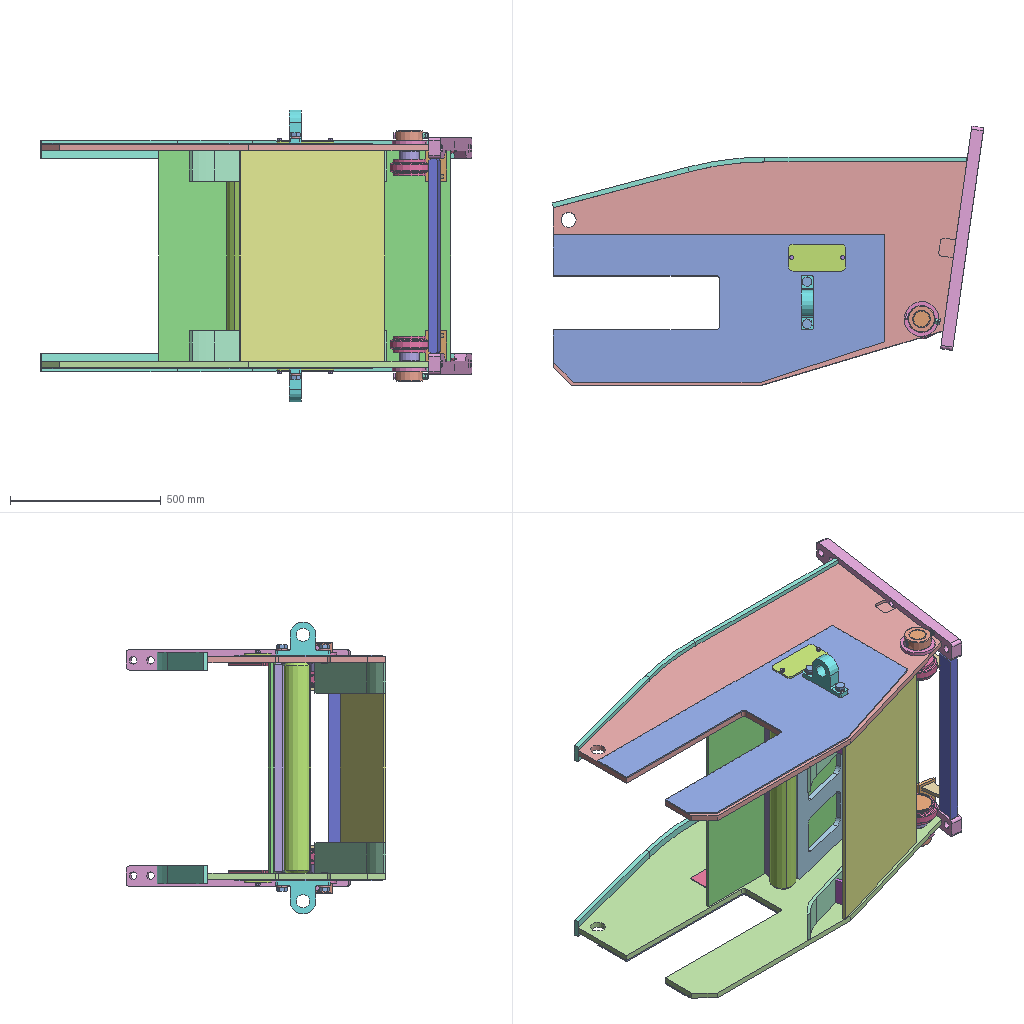Assembly | SolidWorks | 30 different items | 68 placed | box 1432 x 861 x 968 mm
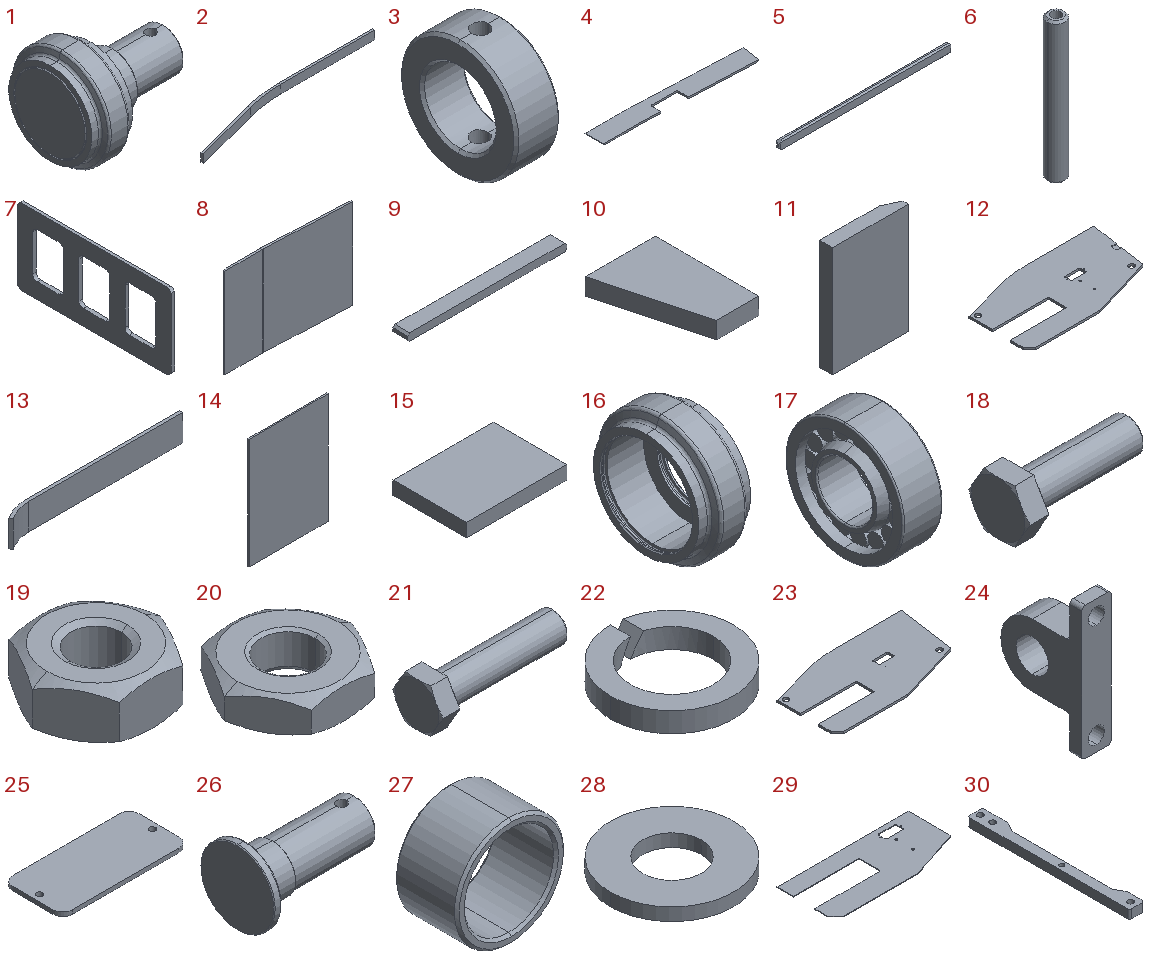Parts list (item | name | quantity | parent item | size | volume | features):
1 | (subassembly) | x2 | - | 150 x 130 x 130 mm | 834716 mm3 | -
2 | - | x2 | - | 1376 x 167.7 x 60 mm | 1336375 mm3 | features Extrusion 1, FlatPattern 1, SheetMetal 1, SolidToSheetMetal 1
3 | - | x2 | - | 34 x 90 x 90 mm | 129031 mm3 | features Chamfer 1, FlatPattern 1, ICE 1, SMBaseFlange 1, SheetMetal 1
4 | - | x2 | - | 922.9 x 138.9 x 10 mm | 889368 mm3 | features Chamfer 1, FlatPattern 1, SMBaseFlange 1, SheetMetal 1
5 | - | x1 | - | 700 x 16 x 37 mm | 375009 mm3 | features Chamfer 2, FlatPattern 1, SMBaseFlange 1, SheetMetal 1
6 | - | x1 | - | 89 x 89 x 700 mm | 3008913 mm3 | features Chamfer 1, ExtruThin 1
7 | - | x1 | - | 16 x 700 x 345 mm | 2478848 mm3 | features Chamfer 2, FlatPattern 1, ICE 1, LPattern 1, SMBaseFlange 1, SheetMetal 1
8 | - | x1 | - | 968.586 x 44.7 x 700 mm | 10744321 mm3 | features Extrusion 1, ICE 1
9 | - | x1 | - | 650 x 60 x 30 mm | 1162320 mm3 | features Chamfer 1, FlatPattern 1, SMBaseFlange 1, SheetMetal 1
10 | - | x2 | - | 50 x 74 x 12 mm | 35520 mm3 | features FlatPattern 1, SMBaseFlange 1, SheetMetal 1
11 | - | x2 | - | 70 x 12 x 102 mm | 80325 mm3 | features Extrusion 1
12 | - | x1 | - | 1372 x 742.1 x 20 mm | 15301514 mm3 | features HoleWzd 2, FlatPattern 1, ICE 1, SMBaseFlange 1, SheetMetal 1
13 | - | x2 | - | 690 x 40 x 102 mm | 847761 mm3 | features Extrusion 1
14 | - | x1 | - | 500 x 8 x 700 mm | 2800000 mm3 | features FlatPattern 1, SMBaseFlange 1, SheetMetal 1
15 | - | x4 | - | 90 x 66 x 12 mm | 71280 mm3 | features FlatPattern 1, SMBaseFlange 1, SheetMetal 1
16 | - | x2 | in 1 | 54 x 130 x 130 mm | 264733 mm3 | features Chamfer 1, Revolution 1
17 | - | x4 | in 1 | 114 x 340 x 340 mm | 5597424 mm3 | features Revolution 3, Fillet 2, CirPattern 1
18 | - | x6 | - | 19.5 x 9.238 x 8 mm | 500.222 mm3 | features RevCut 3, Boss 1, Chamfer 1, Extrusion 1, Fillet 1, LPattern 1
19 | - | x2 | - | 8.083 x 7 x 3.2 mm | 104.299 mm3 | features RevCut 2, Chamfer 1, Extrusion 1, LPattern 1
20 | - | x2 | - | 11.547 x 10 x 3.2 mm | 207.259 mm3 | features RevCut 2, Chamfer 1, Extrusion 1, LPattern 1
21 | - | x4 | - | 92.715 x 34.26 x 29.67 mm | 34696 mm3 | features RevCut 3, Boss 1, Chamfer 1, Extrusion 1, Fillet 1, LPattern 1
22 | - | x8 | - | 19.1 x 19.1 x 3.1 mm | 465.776 mm3 | features Cut 1, Extrusion 1
23 | - | x1 | - | 1372 x 742.1 x 20 mm | 15301514 mm3 | features FlatPattern 2, HoleWzd 2, SheetMetal 2, ICE 1, MirrorSolid 1, SMBaseFlange 1
24 | - | x2 | - | 40 x 109.5 x 180 mm | 329190 mm3 | features Extrusion 1, Fillet 1, ICE 1
25 | - | x2 | - | 190 x 90 x 6 mm | 100678 mm3 | features FlatPattern 1, SMBaseFlange 1, SheetMetal 1
26 | - | x2 | in 1 | 150 x 95 x 95 mm | 409672 mm3 | features Chamfer 1, Fillet 1, ICE 1, Revolution 1
27 | - | x2 | in 1 | 67 x 38.5 x 67 mm | 43406 mm3 | features Chamfer 1, Extrusion 1
28 | - | x2 | - | 116 x 116 x 12 mm | 98310 mm3 | features FlatPattern 1, SMBaseFlange 1, SheetMetal 1
29 | - | x2 | - | 1100 x 490 x 5 mm | 1994925 mm3 | features HoleWzd 2, FlatPattern 1, SMBaseFlange 1, SheetMetal 1
30 | - | x2 | - | 67.5 x 745 x 40 mm | 1428289 mm3 | features HoleWzd 2, FlatPattern 1, SMBaseFlange 1, SheetMetal 1
Mates (type | each side: item.copy, entity, surface, feature):
In the top assembly
Coincident | 12.1 face plane Base-Flange1 | 8.1 face plane Boss-Extrude1
Coincident | 12.1 face plane Base-Flange1 | 30.1 face plane Base-Flange1 | 2 times
Coincident | 12.1 face plane Base-Flange1 | 29.1 face plane Base-Flange1 | 3 times
Coincident | 12.1 face plane Base-Flange1 | 11.1 face plane Boss-Extrude1
Coincident | 30.1 face plane Base-Flange1 | 11.1 edge
DistanceDim | 30.1 face plane Base-Flange1 | 12.1 edge
DistanceDim | 11.1 edge | 30.1 face plane Base-Flange1
Parallel | 30.1 face plane Base-Flange1 | 11.1 face plane Boss-Extrude1
Coincident | 30.1 face plane Base-Flange1 | 2.1 edge
Coincident | 30.1 face plane Base-Flange1 | 2.1 face plane Convert entities1
Coincident | 12.1 face plane Base-Flange1 | 2.1 face plane Convert entities1
Coincident | 12.1 face plane Base-Flange1 | 6.1 face plane Extrude-Thin1 | 2 times
Coincident | 12.1 face plane Base-Flange1 | 5.1 face plane Base-Flange1
Coincident | 5.1 face plane Base-Flange1 | 8.1 face plane Boss-Extrude1
Tangent | 6.1 face cylinder Extrude-Thin1 | 5.1 face plane Base-Flange1
Coincident | 12.1 face plane Base-Flange1 | 4.1 face plane Base-Flange1
Coincident | 30.1 face plane Base-Flange1 | 4.1 face plane Base-Flange1
DistanceDim | 4.1 edge | 8.1 edge
Coincident | 12.1 face plane Base-Flange1 | 7.1 face plane Base-Flange1
Coincident | 6.1 face cylinder Extrude-Thin1 | 7.1 edge
Coincident | 8.1 face plane Boss-Extrude1 | 7.1 edge
Coincident | 12.1 face plane Base-Flange1 | 15.1 face plane Base-Flange1
Coincident | 12.1 face plane Base-Flange1 | 15.2 face plane Base-Flange1
Coincident | 12.1 face plane Base-Flange1 | 14.1 face plane Base-Flange1
DistanceDim | 14.1 face plane Base-Flange1 | 12.1 face plane Base-Flange1
Coincident | 12.1 face plane Base-Flange1 | 14.1 edge
Coincident | 14.1 face plane Base-Flange1 | 15.1 face plane Base-Flange1
Coincident | 14.1 face plane Base-Flange1 | 15.2 face plane Base-Flange1
DistanceDim | 15.2 face plane Base-Flange1 | 14.1 face plane Base-Flange1
DistanceDim | 15.2 face plane Base-Flange1 | 15.1 face plane Base-Flange1
Coincident | 15.2 face plane Base-Flange1 | 13.1 face plane Boss-Extrude1
Coincident | 12.1 face plane Base-Flange1 | 13.1 face plane Boss-Extrude1
Coincident | 12.1 face plane Base-Flange1 | 13.1 edge
Coincident | 30.1 face plane Base-Flange1 | 9.1 face plane Base-Flange1
Coincident | 9.1 face plane Base-Flange1 | 30.2 face plane Base-Flange1
Concentric | 12.1 face cylinder Base-Flange1 | 23.1 face cylinder Mirror1
Coincident | 8.1 face plane Boss-Extrude1 | 23.1 face plane Mirror1
Concentric | 3.1 face cylinder Base-Flange1 | 28.1 face cylinder Base-Flange1
Coincident | 12.1 face plane Base-Flange1 | 28.1 face plane Base-Flange1
Coincident | 29.1 face plane Base-Flange1 | 24.1 face plane Boss-Extrude1
Concentric | 12.1 face cylinder M20 Tapped Hole1 | 24.1 face cylinder Boss-Extrude1 | 2 times
Coincident | 9.1 face plane Base-Flange1 | 10.1 face plane Base-Flange1 | 2 times
DistanceDim | 10.1 face plane Base-Flange1 | 11.1 face plane Boss-Extrude1
DistanceDim | 8.1 edge | 12.1 face plane Base-Flange1
Coincident | 6.1 axis | 5.1 plane
DistanceDim | 8.1 edge | 30.1 face plane Base-Flange1
Coincident | 30.1 face plane Base-Flange1 | 8.1 edge
Concentric | 21.1 face cylinder BaseBody | 22.1 face cylinder Base-Extrude
Coincident | 21.1 face plane BaseHead | 22.1 face plane Base-Extrude
Concentric | 21.2 face cylinder BaseBody | 22.2 face cylinder Base-Extrude
Coincident | 21.2 face plane BaseHead | 22.2 face plane Base-Extrude
Concentric | 24.1 face cylinder Boss-Extrude1 | 21.1 face cylinder BaseBody
Concentric | 24.1 face cylinder Boss-Extrude1 | 21.2 face cylinder BaseBody
Coincident | 24.1 face plane Boss-Extrude1 | 22.2 face plane Base-Extrude
Coincident | 24.1 face plane Boss-Extrude1 | 22.1 face plane Base-Extrude
DistanceDim | 6.1 axis | 12.1 face plane Base-Flange1
Coincident | 12.1 face plane Base-Flange1 | 23.1 face plane Mirror1
Coincident | 29.1 face plane Base-Flange1 | 25.1 face plane Base-Flange1
Concentric | 29.1 face cylinder M8 Tapped Hole1 | 25.1 face cylinder Base-Flange1 | 2 times
Concentric | 22.3 face cylinder Base-Extrude | 18.1 face cylinder BaseBody
Concentric | 22.4 face cylinder Base-Extrude | 18.2 face cylinder BaseBody
Coincident | 22.4 face plane Base-Extrude | 18.2 face plane BaseHead
Coincident | 25.1 face plane Base-Flange1 | 22.4 face plane Base-Extrude
Concentric | 25.1 face cylinder Base-Flange1 | 18.2 face cylinder BaseBody
Concentric | 25.1 face cylinder Base-Flange1 | 18.1 face cylinder BaseBody
Coincident | 25.1 face plane Base-Flange1 | 22.3 face plane Base-Extrude
Coincident | 22.3 face plane Base-Extrude | 18.1 face plane BaseHead
Coincident | 3.1 face plane Base-Flange1 | 28.1 face plane Base-Flange1
Concentric | 3.1 face cylinder Cut-Extrude1 | 18.3 face cylinder BaseBody
Tangent | 3.1 face cylinder Base-Flange1 | 18.3 face plane BaseHead
Concentric | 18.3 face cylinder BaseBody | 19.1 face cylinder BaseNut
Tangent | 3.1 face cylinder Base-Flange1 | 19.1 face plane BaseNut
Concentric | 3.1 face cylinder Base-Flange1 | 26.1 face cylinder Revolve1
Coincident | 12.1 face plane Base-Flange1 | 27.1 face plane Boss-Extrude1
Concentric | 18.3 face cylinder BaseBody | 26.1 face cylinder Cut-Extrude1
Concentric | 12.1 face cylinder Base-Flange1 | 27.1 face cylinder Boss-Extrude1
Concentric | 18.3 face cylinder BaseBody | 20.1 face cylinder BaseNut
Coincident | 19.1 face plane BaseNut | 20.1 face plane BaseNut
In subassembly 1
Concentric | 26.2 face cylinder Revolve1 | 16.1 face cylinder Revolve1
Concentric | 17.1 face cylinder Revolve1 | 17.2 face cylinder Revolve1
Coincident | 17.1 face plane Revolve3 | 17.2 face plane Revolve3
Concentric | 27.2 face cylinder Boss-Extrude1 | 17.2 face cylinder Revolve1
Coincident | 27.2 face plane Boss-Extrude1 | 17.2 face plane Revolve1
Concentric | 26.2 face cylinder Revolve1 | 27.2 face cylinder Boss-Extrude1
Coincident | 17.2 face plane Revolve3 | 16.1 face plane Revolve1
Coincident | 26.2 face plane Revolve1 | 17.1 face plane Revolve3